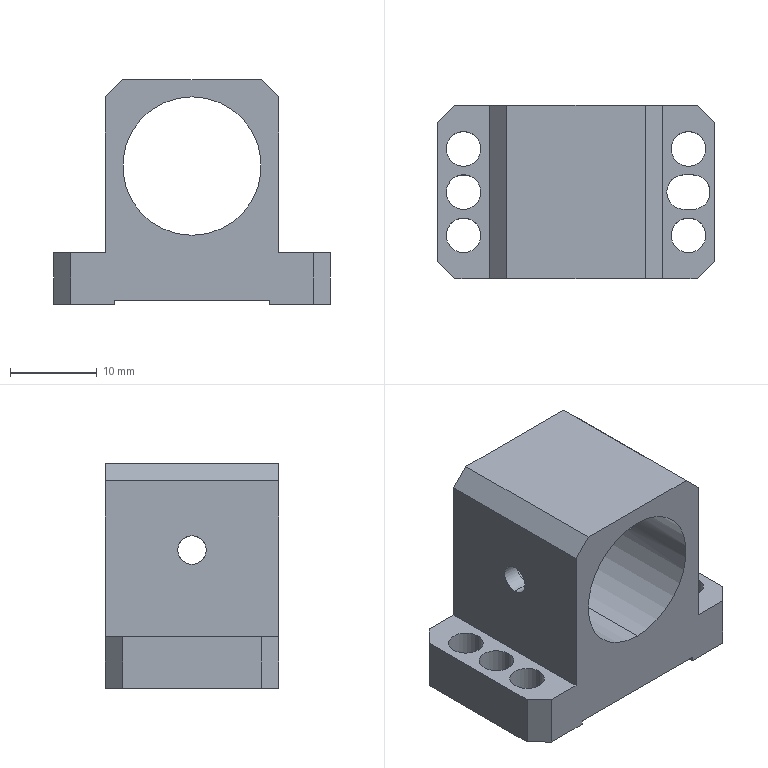NC program | NX | posted with a generic post | part box 32 x 20 x 26 mm
Lines 232 to 1055 of 2499:
(ZLEVEL_PROFILE_COPY_COPY_1 , TOOL : D3)
N444 T03 M6
N446 G54
N448 G17 G0 G90 X-13.314 Y-0.263 B0. C0. S9500 M3
N450 G43 Z30. H3
N452 Z1.
N454 G94 G1 X-13.242 Y-0.319 Z0.995 F1000.
N456 X-13.17 Y-0.373 Z0.99
N458 X-13.003 Y-0.41 Z0.982
N460 X-12.836 Y-0.376 Z0.973
N462 X-12.754 Y-0.316 Z0.967
N464 X-12.683 Y-0.26 Z0.963
N466 X-12.666 Y-0.237 Z0.961
N468 X-12.631 Y-0.154 Z0.956
N470 X-12.637 Y-0.109 Z0.954
N472 X-12.607 Y-0.077 Z0.952
N474 X-12.599 Y-0.036 Z0.949
N476 X-12.601 Y0.078 Z0.943
N478 X-12.63 Y0.152 Z0.939
N480 X-12.664 Y0.235 Z0.935
N482 X-12.828 Y0.372 Z0.923
N484 X-13.038 Y0.408 Z0.912
N486 X-13.209 Y0.353 Z0.903
N488 X-13.334 Y0.238 Z0.894
N490 X-13.402 Y0.082 Z0.885
N492 X-13.399 Y-0.079 Z0.877
N494 X-13.367 Y-0.159 Z0.872
N496 X-13.331 Y-0.242 Z0.867
N498 X-13.317 Y-0.26 Z0.866
N500 X-13.242 Y-0.319 Z0.861
N502 X-13.17 Y-0.373 Z0.856
N504 X-13.003 Y-0.41 Z0.847
N506 X-12.836 Y-0.376 Z0.838
N508 X-12.754 Y-0.316 Z0.833
N510 X-12.683 Y-0.26 Z0.828
N512 X-12.666 Y-0.237 Z0.827
N514 X-12.631 Y-0.154 Z0.822
N516 X-12.637 Y-0.109 Z0.82
N518 X-12.607 Y-0.077 Z0.818
N520 X-12.599 Y-0.036 Z0.815
N522 X-12.601 Y0.078 Z0.809
N524 X-12.63 Y0.152 Z0.805
N526 X-12.664 Y0.235 Z0.8
N528 X-12.828 Y0.372 Z0.789
N530 X-13.038 Y0.408 Z0.778
N532 X-13.209 Y0.353 Z0.769
N534 X-13.334 Y0.238 Z0.76
N536 X-13.402 Y0.082 Z0.751
N538 X-13.399 Y-0.079 Z0.742
N540 X-13.367 Y-0.159 Z0.738
N542 X-13.331 Y-0.242 Z0.733
N544 X-13.317 Y-0.26 Z0.732
N546 X-13.242 Y-0.319 Z0.727
N548 X-13.17 Y-0.373 Z0.722
N550 X-13.003 Y-0.41 Z0.713
N552 X-12.836 Y-0.376 Z0.704
N554 X-12.754 Y-0.316 Z0.699
N556 X-12.683 Y-0.26 Z0.694
N558 X-12.666 Y-0.237 Z0.693
N560 X-12.631 Y-0.154 Z0.688
N562 X-12.637 Y-0.109 Z0.686
N564 X-12.607 Y-0.077 Z0.683
N566 X-12.599 Y-0.036 Z0.681
N568 X-12.601 Y0.078 Z0.675
N570 X-12.63 Y0.152 Z0.671
N572 X-12.664 Y0.235 Z0.666
N574 X-12.828 Y0.372 Z0.655
N576 X-13.038 Y0.408 Z0.644
N578 X-13.209 Y0.353 Z0.635
N580 X-13.334 Y0.238 Z0.626
N582 X-13.402 Y0.082 Z0.617
N584 X-13.399 Y-0.079 Z0.608
N586 X-13.367 Y-0.159 Z0.604
N588 X-13.331 Y-0.242 Z0.599
N590 X-13.317 Y-0.26 Z0.598
N592 X-13.242 Y-0.319 Z0.593
N594 X-13.17 Y-0.373 Z0.588
N596 X-13.003 Y-0.41 Z0.579
N598 X-12.836 Y-0.376 Z0.57
N600 X-12.754 Y-0.316 Z0.565
N602 X-12.683 Y-0.26 Z0.56
N604 X-12.666 Y-0.237 Z0.559
N606 X-12.631 Y-0.154 Z0.554
N608 X-12.637 Y-0.109 Z0.552
N610 X-12.607 Y-0.077 Z0.549
N612 X-12.599 Y-0.036 Z0.547
N614 X-12.601 Y0.078 Z0.541
N616 X-12.63 Y0.152 Z0.537
N618 X-12.664 Y0.235 Z0.532
N620 X-12.828 Y0.372 Z0.521
N622 X-13.038 Y0.408 Z0.51
N624 X-13.209 Y0.353 Z0.5
N626 X-13.334 Y0.238 Z0.492
N628 X-13.402 Y0.082 Z0.483
N630 X-13.399 Y-0.079 Z0.474
N632 X-13.367 Y-0.159 Z0.47
N634 X-13.331 Y-0.242 Z0.465
N636 X-13.317 Y-0.26 Z0.464
N638 X-13.242 Y-0.319 Z0.459
N640 X-13.17 Y-0.373 Z0.454
N642 X-13.003 Y-0.41 Z0.445
N644 X-12.836 Y-0.376 Z0.436
N646 X-12.754 Y-0.316 Z0.431
N648 X-12.683 Y-0.26 Z0.426
N650 X-12.666 Y-0.237 Z0.425
N652 X-12.631 Y-0.154 Z0.42
N654 X-12.637 Y-0.109 Z0.418
N656 X-12.607 Y-0.077 Z0.415
N658 X-12.599 Y-0.036 Z0.413
N660 X-12.601 Y0.078 Z0.407
N662 X-12.63 Y0.152 Z0.403
N664 X-12.664 Y0.235 Z0.398
N666 X-12.828 Y0.372 Z0.387
N668 X-13.038 Y0.408 Z0.376
N670 X-13.209 Y0.353 Z0.366
N672 X-13.334 Y0.238 Z0.358
N674 X-13.402 Y0.082 Z0.349
N676 X-13.399 Y-0.079 Z0.34
N678 X-13.367 Y-0.159 Z0.336
N680 X-13.331 Y-0.242 Z0.331
N682 X-13.317 Y-0.26 Z0.33
N684 X-13.242 Y-0.319 Z0.325
N686 X-13.17 Y-0.373 Z0.32
N688 X-13.003 Y-0.41 Z0.311
N690 X-12.836 Y-0.376 Z0.302
N692 X-12.754 Y-0.316 Z0.297
N694 X-12.683 Y-0.26 Z0.292
N696 X-12.666 Y-0.237 Z0.291
N698 X-12.631 Y-0.154 Z0.286
N700 X-12.637 Y-0.109 Z0.283
N702 X-12.607 Y-0.077 Z0.281
N704 X-12.599 Y-0.036 Z0.279
N706 X-12.601 Y0.078 Z0.273
N708 X-12.63 Y0.152 Z0.269
N710 X-12.664 Y0.235 Z0.264
N712 X-12.828 Y0.372 Z0.253
N714 X-13.038 Y0.408 Z0.242
N716 X-13.209 Y0.353 Z0.232
N718 X-13.334 Y0.238 Z0.223
N720 X-13.402 Y0.082 Z0.215
N722 X-13.399 Y-0.079 Z0.206
N724 X-13.367 Y-0.159 Z0.202
N726 X-13.331 Y-0.242 Z0.197
N728 X-13.317 Y-0.26 Z0.196
N730 X-13.242 Y-0.319 Z0.191
N732 X-13.17 Y-0.373 Z0.186
N734 X-13.003 Y-0.41 Z0.177
N736 X-12.836 Y-0.376 Z0.168
N738 X-12.754 Y-0.316 Z0.163
N740 X-12.683 Y-0.26 Z0.158
N742 X-12.666 Y-0.237 Z0.156
N744 X-12.631 Y-0.154 Z0.152
N746 X-12.637 Y-0.109 Z0.149
N748 X-12.607 Y-0.077 Z0.147
N750 X-12.599 Y-0.036 Z0.145
N752 X-12.601 Y0.078 Z0.139
N754 X-12.63 Y0.152 Z0.135
N756 X-12.664 Y0.235 Z0.13
N758 X-12.828 Y0.372 Z0.119
N760 X-13.038 Y0.408 Z0.108
N762 X-13.209 Y0.353 Z0.098
N764 X-13.334 Y0.238 Z0.089
N766 X-13.402 Y0.082 Z0.08
N768 X-13.399 Y-0.079 Z0.072
N770 X-13.367 Y-0.159 Z0.067
N772 X-13.331 Y-0.242 Z0.063
N774 X-13.317 Y-0.26 Z0.062
N776 X-13.242 Y-0.319 Z0.057
N778 X-13.17 Y-0.373 Z0.052
N780 X-13.003 Y-0.41 Z0.043
N782 X-12.836 Y-0.376 Z0.034
N784 X-12.754 Y-0.316 Z0.029
N786 X-12.683 Y-0.26 Z0.024
N788 X-12.666 Y-0.237 Z0.022
N790 X-12.631 Y-0.154 Z0.018
N792 X-12.637 Y-0.109 Z0.015
N794 X-12.607 Y-0.077 Z0.013
N796 X-12.599 Y-0.036 Z0.011
N798 X-12.601 Y0.078 Z0.005
N800 X-12.63 Y0.152 Z0.001
N802 X-12.664 Y0.235 Z-0.004
N804 X-12.828 Y0.372 Z-0.015
N806 X-13.038 Y0.408 Z-0.026
N808 X-13.209 Y0.353 Z-0.036
N810 X-13.334 Y0.238 Z-0.045
N812 X-13.402 Y0.082 Z-0.054
N814 X-13.399 Y-0.079 Z-0.062
N816 X-13.367 Y-0.159 Z-0.067
N818 X-13.331 Y-0.242 Z-0.071
N820 X-13.317 Y-0.26 Z-0.073
N822 X-13.242 Y-0.319 Z-0.078
N824 X-13.17 Y-0.373 Z-0.082
N826 X-13.003 Y-0.41 Z-0.091
N828 X-12.836 Y-0.376 Z-0.1
N830 X-12.754 Y-0.316 Z-0.106
N832 X-12.683 Y-0.26 Z-0.11
N834 X-12.666 Y-0.237 Z-0.112
N836 X-12.631 Y-0.154 Z-0.116
N838 X-12.637 Y-0.109 Z-0.119
N840 X-12.607 Y-0.077 Z-0.121
N842 X-12.599 Y-0.036 Z-0.123
N844 X-12.601 Y0.078 Z-0.129
N846 X-12.63 Y0.152 Z-0.134
N848 X-12.664 Y0.235 Z-0.138
N850 X-12.828 Y0.372 Z-0.149
N852 X-13.038 Y0.408 Z-0.161
N854 X-13.209 Y0.353 Z-0.17
N856 X-13.334 Y0.238 Z-0.179
N858 X-13.402 Y0.082 Z-0.188
N860 X-13.399 Y-0.079 Z-0.196
N862 X-13.372 Y-0.146 Z-0.2
N864 X-13.367 Y-0.159 F1200.
N866 G3 X-12.631 Y-0.154 R0.4
N868 G1 X-12.641 Y-0.125
N870 X-12.632 Y-0.096
N872 X-12.607 Y-0.077
N874 G3 X-13.372 Y-0.146 R-0.4
N876 G1 X-13.319 Y-0.228 Z-0.21
N878 X-13.269 Y-0.286 Z-0.219
N880 X-13.224 Y-0.322 Z-0.225
N882 X-13.139 Y-0.366 Z-0.235
N884 X-13.095 Y-0.381 Z-0.24
N886 X-13.066 Y-0.387 Z-0.243
N888 X-13.007 Y-0.392 Z-0.25
N890 X-12.912 Y-0.382 Z-0.26
N892 X-12.868 Y-0.369 Z-0.265
N894 X-12.84 Y-0.358 Z-0.268
N896 X-12.788 Y-0.33 Z-0.275
N898 X-12.715 Y-0.269 Z-0.285
N900 X-12.685 Y-0.234 Z-0.29
N902 X-12.668 Y-0.209 Z-0.293
N904 X-12.64 Y-0.156 Z-0.3
N906 X-12.613 Y-0.066 Z-0.31
N908 X-12.608 Y-0.021 Z-0.315
N910 X-12.607 Y0.009 Z-0.318
N912 X-12.614 Y0.068 Z-0.325
N914 X-12.642 Y0.159 Z-0.335
N916 X-12.663 Y0.2 Z-0.34
N918 X-12.679 Y0.225 Z-0.343
N920 X-12.717 Y0.271 Z-0.35
N922 X-12.789 Y0.33 Z-0.36
N924 X-12.828 Y0.352 Z-0.365
N926 X-12.856 Y0.365 Z-0.368
N928 X-12.915 Y0.383 Z-0.375
N930 X-12.974 Y0.391 Z-0.381
N932 X-13.031 Z-0.388
N934 X-13.089 Y0.383 Z-0.394
N936 X-13.145 Y0.373 Z-0.4
N938 G3 X-13.372 Y-0.146 R0.4
N940 G1 X-13.319 Y-0.228 Z-0.41
N942 X-13.269 Y-0.286 Z-0.419
N944 X-13.224 Y-0.322 Z-0.425
N946 X-13.139 Y-0.366 Z-0.435
N948 X-13.095 Y-0.381 Z-0.44
N950 X-13.066 Y-0.387 Z-0.443
N952 X-13.007 Y-0.392 Z-0.45
N954 X-12.912 Y-0.382 Z-0.46
N956 X-12.868 Y-0.369 Z-0.465
N958 X-12.84 Y-0.358 Z-0.468
N960 X-12.788 Y-0.33 Z-0.475
N962 X-12.715 Y-0.269 Z-0.485
N964 X-12.685 Y-0.234 Z-0.49
N966 X-12.668 Y-0.209 Z-0.493
N968 X-12.64 Y-0.156 Z-0.5
N970 X-12.613 Y-0.066 Z-0.51
N972 X-12.608 Y-0.021 Z-0.515
N974 X-12.607 Y0.009 Z-0.518
N976 X-12.614 Y0.068 Z-0.525
N978 X-12.642 Y0.159 Z-0.535
N980 X-12.663 Y0.2 Z-0.54
N982 X-12.679 Y0.225 Z-0.543
N984 X-12.717 Y0.271 Z-0.55
N986 X-12.789 Y0.33 Z-0.56
N988 X-12.828 Y0.352 Z-0.565
N990 X-12.856 Y0.365 Z-0.568
N992 X-12.915 Y0.383 Z-0.575
N994 X-12.974 Y0.391 Z-0.581
N996 X-13.031 Z-0.588
N998 X-13.089 Y0.383 Z-0.594
N1000 X-13.145 Y0.373 Z-0.6
N1002 G3 X-13.372 Y-0.146 R0.4
N1004 G1 X-13.319 Y-0.228 Z-0.61
N1006 X-13.269 Y-0.286 Z-0.619
N1008 X-13.224 Y-0.322 Z-0.625
N1010 X-13.139 Y-0.366 Z-0.635
N1012 X-13.095 Y-0.381 Z-0.64
N1014 X-13.066 Y-0.387 Z-0.643
N1016 X-13.007 Y-0.392 Z-0.65
N1018 X-12.912 Y-0.382 Z-0.66
N1020 X-12.868 Y-0.369 Z-0.665
N1022 X-12.84 Y-0.358 Z-0.668
N1024 X-12.788 Y-0.33 Z-0.675
N1026 X-12.715 Y-0.269 Z-0.685
N1028 X-12.685 Y-0.234 Z-0.69
N1030 X-12.668 Y-0.209 Z-0.693
N1032 X-12.64 Y-0.156 Z-0.7
N1034 X-12.613 Y-0.066 Z-0.71
N1036 X-12.608 Y-0.021 Z-0.715
N1038 X-12.607 Y0.009 Z-0.718
N1040 X-12.614 Y0.068 Z-0.725
N1042 X-12.642 Y0.159 Z-0.735
N1044 X-12.663 Y0.2 Z-0.74
N1046 X-12.679 Y0.225 Z-0.743
N1048 X-12.717 Y0.271 Z-0.75
N1050 X-12.789 Y0.33 Z-0.76
N1052 X-12.828 Y0.352 Z-0.765
N1054 X-12.856 Y0.365 Z-0.768
N1056 X-12.915 Y0.383 Z-0.775
N1058 X-12.974 Y0.391 Z-0.781
N1060 X-13.031 Z-0.788
N1062 X-13.089 Y0.383 Z-0.794
N1064 X-13.145 Y0.373 Z-0.8
N1066 G3 X-13.372 Y-0.146 R0.4
N1068 G1 X-13.319 Y-0.228 Z-0.81
N1070 X-13.269 Y-0.286 Z-0.819
N1072 X-13.224 Y-0.322 Z-0.825
N1074 X-13.139 Y-0.366 Z-0.835
N1076 X-13.095 Y-0.381 Z-0.84
N1078 X-13.066 Y-0.387 Z-0.843
N1080 X-13.007 Y-0.392 Z-0.85
N1082 X-12.912 Y-0.382 Z-0.86
N1084 X-12.868 Y-0.369 Z-0.865
N1086 X-12.84 Y-0.358 Z-0.868
N1088 X-12.788 Y-0.33 Z-0.875
N1090 X-12.715 Y-0.269 Z-0.885
N1092 X-12.685 Y-0.234 Z-0.89
N1094 X-12.668 Y-0.209 Z-0.893
N1096 X-12.64 Y-0.156 Z-0.9
N1098 X-12.613 Y-0.066 Z-0.91
N1100 X-12.608 Y-0.021 Z-0.915
N1102 X-12.607 Y0.009 Z-0.918
N1104 X-12.614 Y0.068 Z-0.925
N1106 X-12.642 Y0.159 Z-0.935
N1108 X-12.663 Y0.2 Z-0.94
N1110 X-12.679 Y0.225 Z-0.943
N1112 X-12.717 Y0.271 Z-0.95
N1114 X-12.789 Y0.33 Z-0.96
N1116 X-12.828 Y0.352 Z-0.965
N1118 X-12.856 Y0.365 Z-0.968
N1120 X-12.915 Y0.383 Z-0.975
N1122 X-12.974 Y0.391 Z-0.981
N1124 X-13.031 Z-0.988
N1126 X-13.089 Y0.383 Z-0.994
N1128 X-13.145 Y0.373 Z-1.
N1130 G3 X-13.372 Y-0.146 R0.4
N1132 G1 X-13.319 Y-0.228 Z-1.01
N1134 X-13.269 Y-0.286 Z-1.019
N1136 X-13.224 Y-0.322 Z-1.025
N1138 X-13.139 Y-0.366 Z-1.035
N1140 X-13.095 Y-0.381 Z-1.04
N1142 X-13.066 Y-0.387 Z-1.043
N1144 X-13.007 Y-0.392 Z-1.05
N1146 X-12.912 Y-0.382 Z-1.06
N1148 X-12.868 Y-0.369 Z-1.065
N1150 X-12.84 Y-0.358 Z-1.068
N1152 X-12.788 Y-0.33 Z-1.075
N1154 X-12.715 Y-0.269 Z-1.085
N1156 X-12.685 Y-0.234 Z-1.09
N1158 X-12.668 Y-0.209 Z-1.093
N1160 X-12.64 Y-0.156 Z-1.1
N1162 X-12.613 Y-0.066 Z-1.11
N1164 X-12.608 Y-0.021 Z-1.115
N1166 X-12.607 Y0.009 Z-1.118
N1168 X-12.614 Y0.068 Z-1.125
N1170 X-12.642 Y0.159 Z-1.135
N1172 X-12.663 Y0.2 Z-1.14
N1174 X-12.679 Y0.225 Z-1.143
N1176 X-12.717 Y0.271 Z-1.15
N1178 X-12.789 Y0.33 Z-1.16
N1180 X-12.828 Y0.352 Z-1.165
N1182 X-12.856 Y0.365 Z-1.168
N1184 X-12.915 Y0.383 Z-1.175
N1186 X-12.974 Y0.391 Z-1.181
N1188 X-13.031 Z-1.188
N1190 X-13.089 Y0.383 Z-1.194
N1192 X-13.145 Y0.373 Z-1.2
N1194 G3 X-13.372 Y-0.146 R0.4
N1196 G1 X-13.319 Y-0.228 Z-1.21
N1198 X-13.269 Y-0.286 Z-1.219
N1200 X-13.224 Y-0.322 Z-1.225
N1202 X-13.139 Y-0.366 Z-1.235
N1204 X-13.095 Y-0.381 Z-1.24
N1206 X-13.066 Y-0.387 Z-1.243
N1208 X-13.007 Y-0.392 Z-1.25
N1210 X-12.912 Y-0.382 Z-1.26
N1212 X-12.868 Y-0.369 Z-1.265
N1214 X-12.84 Y-0.358 Z-1.268
N1216 X-12.788 Y-0.33 Z-1.275
N1218 X-12.715 Y-0.269 Z-1.285
N1220 X-12.685 Y-0.234 Z-1.29
N1222 X-12.668 Y-0.209 Z-1.293
N1224 X-12.64 Y-0.156 Z-1.3
N1226 X-12.613 Y-0.066 Z-1.31
N1228 X-12.608 Y-0.021 Z-1.315
N1230 Y0.009 Z-1.318
N1232 X-12.614 Y0.068 Z-1.325
N1234 X-12.642 Y0.159 Z-1.335
N1236 X-12.663 Y0.2 Z-1.34
N1238 X-12.679 Y0.225 Z-1.343
N1240 X-12.717 Y0.271 Z-1.35
N1242 X-12.789 Y0.33 Z-1.36
N1244 X-12.828 Y0.352 Z-1.365
N1246 X-12.856 Y0.365 Z-1.368
N1248 X-12.915 Y0.383 Z-1.375
N1250 X-12.974 Y0.391 Z-1.381
N1252 X-13.031 Z-1.388
N1254 X-13.089 Y0.383 Z-1.394
N1256 X-13.145 Y0.373 Z-1.4
N1258 G3 X-13.372 Y-0.146 R0.4
N1260 G1 X-13.319 Y-0.228 Z-1.41
N1262 X-13.269 Y-0.286 Z-1.419
N1264 X-13.224 Y-0.322 Z-1.425
N1266 X-13.139 Y-0.366 Z-1.435
N1268 X-13.095 Y-0.38 Z-1.44
N1270 X-13.066 Y-0.387 Z-1.443
N1272 X-13.007 Y-0.392 Z-1.45
N1274 X-12.912 Y-0.382 Z-1.46
N1276 X-12.868 Y-0.369 Z-1.465
N1278 X-12.84 Y-0.358 Z-1.468
N1280 X-12.788 Y-0.33 Z-1.475
N1282 X-12.715 Y-0.269 Z-1.485
N1284 X-12.685 Y-0.234 Z-1.49
N1286 X-12.668 Y-0.209 Z-1.493
N1288 X-12.64 Y-0.156 Z-1.5
N1290 X-12.613 Y-0.066 Z-1.51
N1292 X-12.608 Y-0.021 Z-1.515
N1294 Y0.009 Z-1.518
N1296 X-12.614 Y0.068 Z-1.525
N1298 X-12.642 Y0.159 Z-1.535
N1300 X-12.663 Y0.2 Z-1.54
N1302 X-12.679 Y0.225 Z-1.543
N1304 X-12.717 Y0.271 Z-1.55
N1306 X-12.789 Y0.33 Z-1.56
N1308 X-12.828 Y0.352 Z-1.565
N1310 X-12.856 Y0.365 Z-1.568
N1312 X-12.915 Y0.383 Z-1.575
N1314 X-12.974 Y0.391 Z-1.581
N1316 X-13.031 Z-1.588
N1318 X-13.089 Y0.383 Z-1.594
N1320 X-13.145 Y0.373 Z-1.6
N1322 G3 X-13.372 Y-0.146 R0.4
N1324 G1 X-13.319 Y-0.228 Z-1.61
N1326 X-13.269 Y-0.286 Z-1.619
N1328 X-13.224 Y-0.322 Z-1.625
N1330 X-13.139 Y-0.366 Z-1.635
N1332 X-13.095 Y-0.38 Z-1.64
N1334 X-13.066 Y-0.387 Z-1.643
N1336 X-13.007 Y-0.392 Z-1.65
N1338 X-12.912 Y-0.382 Z-1.66
N1340 X-12.868 Y-0.369 Z-1.665
N1342 X-12.84 Y-0.358 Z-1.668
N1344 X-12.788 Y-0.33 Z-1.675
N1346 X-12.715 Y-0.269 Z-1.685
N1348 X-12.685 Y-0.234 Z-1.69
N1350 X-12.668 Y-0.209 Z-1.693
N1352 X-12.64 Y-0.156 Z-1.7
N1354 X-12.613 Y-0.066 Z-1.71
N1356 X-12.608 Y-0.021 Z-1.715
N1358 Y0.009 Z-1.718
N1360 X-12.614 Y0.068 Z-1.725
N1362 X-12.642 Y0.159 Z-1.735
N1364 X-12.663 Y0.2 Z-1.74
N1366 X-12.679 Y0.225 Z-1.743
N1368 X-12.717 Y0.271 Z-1.75
N1370 X-12.789 Y0.33 Z-1.76
N1372 X-12.828 Y0.352 Z-1.765
N1374 X-12.856 Y0.365 Z-1.768
N1376 X-12.915 Y0.383 Z-1.775
N1378 X-12.974 Y0.391 Z-1.781
N1380 X-13.031 Z-1.788
N1382 X-13.089 Y0.383 Z-1.794
N1384 X-13.145 Y0.373 Z-1.8
N1386 G3 X-13.372 Y-0.146 R0.4
N1388 G1 X-13.319 Y-0.228 Z-1.81
N1390 X-13.269 Y-0.286 Z-1.819
N1392 X-13.224 Y-0.322 Z-1.825
N1394 X-13.139 Y-0.366 Z-1.835
N1396 X-13.095 Y-0.38 Z-1.84
N1398 X-13.066 Y-0.387 Z-1.843
N1400 X-13.007 Y-0.392 Z-1.85
N1402 X-12.912 Y-0.382 Z-1.86
N1404 X-12.868 Y-0.369 Z-1.865
N1406 X-12.84 Y-0.358 Z-1.868
N1408 X-12.788 Y-0.33 Z-1.875
N1410 X-12.715 Y-0.269 Z-1.885
N1412 X-12.685 Y-0.234 Z-1.89
N1414 X-12.668 Y-0.209 Z-1.893
N1416 X-12.64 Y-0.156 Z-1.9
N1418 X-12.613 Y-0.066 Z-1.91
N1420 X-12.608 Y-0.021 Z-1.915
N1422 Y0.009 Z-1.918
N1424 X-12.614 Y0.068 Z-1.925
N1426 X-12.642 Y0.159 Z-1.935
N1428 X-12.663 Y0.2 Z-1.94
N1430 X-12.679 Y0.225 Z-1.943
N1432 X-12.717 Y0.271 Z-1.95
N1434 X-12.789 Y0.33 Z-1.96
N1436 X-12.828 Y0.352 Z-1.965
N1438 X-12.856 Y0.365 Z-1.968
N1440 X-12.915 Y0.383 Z-1.975
N1442 X-12.974 Y0.391 Z-1.981
N1444 X-13.031 Z-1.988
N1446 X-13.089 Y0.383 Z-1.994
N1448 X-13.145 Y0.373 Z-2.
N1450 G3 X-13.372 Y-0.146 R0.4
N1452 G1 X-13.319 Y-0.228 Z-2.01
N1454 X-13.269 Y-0.286 Z-2.019
N1456 X-13.224 Y-0.322 Z-2.025
N1458 X-13.139 Y-0.366 Z-2.035
N1460 X-13.095 Y-0.38 Z-2.04
N1462 X-13.066 Y-0.387 Z-2.043
N1464 X-13.007 Y-0.392 Z-2.05
N1466 X-12.912 Y-0.382 Z-2.06
N1468 X-12.868 Y-0.369 Z-2.065
N1470 X-12.84 Y-0.358 Z-2.068
N1472 X-12.788 Y-0.33 Z-2.075
N1474 X-12.715 Y-0.269 Z-2.085
N1476 X-12.685 Y-0.234 Z-2.09
N1478 X-12.668 Y-0.209 Z-2.093
N1480 X-12.64 Y-0.156 Z-2.1
N1482 X-12.613 Y-0.066 Z-2.11
N1484 X-12.608 Y-0.021 Z-2.115
N1486 Y0.009 Z-2.118
N1488 X-12.614 Y0.068 Z-2.125
N1490 X-12.642 Y0.159 Z-2.135
N1492 X-12.663 Y0.2 Z-2.14
N1494 X-12.679 Y0.225 Z-2.143
N1496 X-12.717 Y0.271 Z-2.15
N1498 X-12.789 Y0.33 Z-2.16
N1500 X-12.828 Y0.352 Z-2.165
N1502 X-12.856 Y0.365 Z-2.168
N1504 X-12.915 Y0.383 Z-2.175
N1506 X-12.974 Y0.391 Z-2.181
N1508 X-13.031 Z-2.188
N1510 X-13.089 Y0.383 Z-2.194
N1512 X-13.145 Y0.373 Z-2.2
N1514 G3 X-13.372 Y-0.146 R0.4
N1516 G1 X-13.319 Y-0.228 Z-2.21
N1518 X-13.269 Y-0.286 Z-2.219
N1520 X-13.224 Y-0.322 Z-2.225
N1522 X-13.139 Y-0.366 Z-2.235
N1524 X-13.095 Y-0.38 Z-2.24
N1526 X-13.066 Y-0.387 Z-2.243
N1528 X-13.007 Y-0.392 Z-2.25
N1530 X-12.912 Y-0.382 Z-2.26
N1532 X-12.868 Y-0.369 Z-2.265
N1534 X-12.84 Y-0.358 Z-2.268
N1536 X-12.788 Y-0.33 Z-2.275
N1538 X-12.715 Y-0.269 Z-2.285
N1540 X-12.685 Y-0.234 Z-2.29
N1542 X-12.668 Y-0.209 Z-2.293
N1544 X-12.64 Y-0.156 Z-2.3
N1546 X-12.613 Y-0.066 Z-2.31
N1548 X-12.608 Y-0.021 Z-2.315
N1550 Y0.009 Z-2.318
N1552 X-12.614 Y0.068 Z-2.325
N1554 X-12.642 Y0.159 Z-2.335
N1556 X-12.663 Y0.2 Z-2.34
N1558 X-12.679 Y0.225 Z-2.343
N1560 X-12.717 Y0.271 Z-2.35
N1562 X-12.789 Y0.33 Z-2.36
N1564 X-12.828 Y0.352 Z-2.365
N1566 X-12.856 Y0.365 Z-2.368
N1568 X-12.915 Y0.383 Z-2.375
N1570 X-12.974 Y0.391 Z-2.381
N1572 X-13.031 Z-2.388
N1574 X-13.089 Y0.383 Z-2.394
N1576 X-13.145 Y0.373 Z-2.4
N1578 G3 X-13.372 Y-0.146 R0.4
N1580 G1 X-13.319 Y-0.228 Z-2.41
N1582 X-13.269 Y-0.286 Z-2.419
N1584 X-13.224 Y-0.322 Z-2.425
N1586 X-13.139 Y-0.366 Z-2.435
N1588 X-13.095 Y-0.38 Z-2.44
N1590 X-13.066 Y-0.387 Z-2.443
N1592 X-13.007 Y-0.392 Z-2.45
N1594 X-12.912 Y-0.382 Z-2.46
N1596 X-12.868 Y-0.369 Z-2.465
N1598 X-12.84 Y-0.358 Z-2.468
N1600 X-12.788 Y-0.33 Z-2.475
N1602 X-12.715 Y-0.269 Z-2.485
N1604 X-12.685 Y-0.234 Z-2.49
N1606 X-12.668 Y-0.209 Z-2.493
N1608 X-12.64 Y-0.156 Z-2.5
N1610 X-12.613 Y-0.066 Z-2.51
N1612 X-12.608 Y-0.021 Z-2.515
N1614 Y0.009 Z-2.518
N1616 X-12.614 Y0.068 Z-2.525
N1618 X-12.642 Y0.159 Z-2.535
N1620 X-12.663 Y0.2 Z-2.54
N1622 X-12.679 Y0.225 Z-2.543
N1624 X-12.717 Y0.271 Z-2.55
N1626 X-12.789 Y0.33 Z-2.56
N1628 X-12.828 Y0.352 Z-2.565
N1630 X-12.856 Y0.365 Z-2.568
N1632 X-12.915 Y0.383 Z-2.575
N1634 X-12.974 Y0.391 Z-2.581
N1636 X-13.031 Z-2.588
N1638 X-13.089 Y0.383 Z-2.594
N1640 X-13.145 Y0.373 Z-2.6
N1642 G3 X-13.372 Y-0.146 R0.4
N1644 G1 X-13.319 Y-0.228 Z-2.61
N1646 X-13.269 Y-0.286 Z-2.619
N1648 X-13.224 Y-0.322 Z-2.625
N1650 X-13.139 Y-0.366 Z-2.635
N1652 X-13.095 Y-0.38 Z-2.64
N1654 X-13.066 Y-0.387 Z-2.643
N1656 X-13.007 Y-0.392 Z-2.65
N1658 X-12.912 Y-0.382 Z-2.66
N1660 X-12.868 Y-0.369 Z-2.665
N1662 X-12.84 Y-0.358 Z-2.668
N1664 X-12.788 Y-0.33 Z-2.675
N1666 X-12.715 Y-0.269 Z-2.685
N1668 X-12.685 Y-0.234 Z-2.69
N1670 X-12.668 Y-0.209 Z-2.693
N1672 X-12.64 Y-0.156 Z-2.7
N1674 X-12.613 Y-0.066 Z-2.71
N1676 X-12.608 Y-0.021 Z-2.715
N1678 Y0.009 Z-2.718
N1680 X-12.614 Y0.068 Z-2.725
N1682 X-12.642 Y0.159 Z-2.735
N1684 X-12.663 Y0.2 Z-2.74
N1686 X-12.679 Y0.225 Z-2.743
N1688 X-12.717 Y0.271 Z-2.75
N1690 X-12.789 Y0.33 Z-2.76
N1692 X-12.828 Y0.352 Z-2.765
N1694 X-12.856 Y0.365 Z-2.768
N1696 X-12.915 Y0.383 Z-2.775
N1698 X-12.974 Y0.391 Z-2.781
N1700 X-13.031 Z-2.788
N1702 X-13.089 Y0.383 Z-2.794
N1704 X-13.145 Y0.373 Z-2.8
N1706 G3 X-13.372 Y-0.146 R0.4
N1708 G1 X-13.319 Y-0.228 Z-2.81
N1710 X-13.269 Y-0.286 Z-2.819
N1712 X-13.224 Y-0.322 Z-2.825
N1714 X-13.139 Y-0.366 Z-2.835
N1716 X-13.095 Y-0.38 Z-2.84
N1718 X-13.066 Y-0.387 Z-2.843
N1720 X-13.007 Y-0.392 Z-2.85
N1722 X-12.912 Y-0.382 Z-2.86
N1724 X-12.868 Y-0.369 Z-2.865
N1726 X-12.84 Y-0.358 Z-2.868
N1728 X-12.788 Y-0.33 Z-2.875
N1730 X-12.715 Y-0.269 Z-2.885
N1732 X-12.685 Y-0.234 Z-2.89
N1734 X-12.668 Y-0.209 Z-2.893
N1736 X-12.64 Y-0.156 Z-2.9
N1738 X-12.613 Y-0.066 Z-2.91
N1740 X-12.608 Y-0.021 Z-2.915
N1742 Y0.009 Z-2.918
N1744 X-12.614 Y0.068 Z-2.925
N1746 X-12.642 Y0.159 Z-2.935
N1748 X-12.663 Y0.2 Z-2.94
N1750 X-12.679 Y0.225 Z-2.943
N1752 X-12.717 Y0.271 Z-2.95
N1754 X-12.789 Y0.33 Z-2.96
N1756 X-12.828 Y0.352 Z-2.965
N1758 X-12.856 Y0.365 Z-2.968
N1760 X-12.915 Y0.383 Z-2.975
N1762 X-12.974 Y0.391 Z-2.981
N1764 X-13.031 Z-2.988
N1766 X-13.089 Y0.383 Z-2.994
N1768 X-13.145 Y0.373 Z-3.
N1770 G3 X-13.372 Y-0.146 R0.4
N1772 G1 X-13.319 Y-0.228 Z-3.01
N1774 X-13.269 Y-0.286 Z-3.019
N1776 X-13.224 Y-0.322 Z-3.025
N1778 X-13.139 Y-0.366 Z-3.035
N1780 X-13.095 Y-0.38 Z-3.04
N1782 X-13.066 Y-0.387 Z-3.043
N1784 X-13.007 Y-0.392 Z-3.05
N1786 X-12.912 Y-0.382 Z-3.06
N1788 X-12.868 Y-0.369 Z-3.065
N1790 X-12.84 Y-0.358 Z-3.068
N1792 X-12.788 Y-0.33 Z-3.075
N1794 X-12.715 Y-0.269 Z-3.085
N1796 X-12.685 Y-0.234 Z-3.09
N1798 X-12.668 Y-0.209 Z-3.093
N1800 X-12.64 Y-0.156 Z-3.1
N1802 X-12.613 Y-0.066 Z-3.11
N1804 X-12.608 Y-0.021 Z-3.115
N1806 Y0.009 Z-3.118
N1808 X-12.614 Y0.068 Z-3.125
N1810 X-12.642 Y0.159 Z-3.135
N1812 X-12.663 Y0.2 Z-3.14
N1814 X-12.679 Y0.225 Z-3.143
N1816 X-12.717 Y0.271 Z-3.15
N1818 X-12.789 Y0.33 Z-3.16
N1820 X-12.828 Y0.352 Z-3.165
N1822 X-12.856 Y0.365 Z-3.168
N1824 X-12.915 Y0.383 Z-3.175
N1826 X-12.974 Y0.391 Z-3.181
N1828 X-13.031 Z-3.188
N1830 X-13.089 Y0.383 Z-3.194
N1832 X-13.145 Y0.373 Z-3.2
N1834 G3 X-13.372 Y-0.146 R0.4
N1836 G1 X-13.319 Y-0.228 Z-3.21
N1838 X-13.269 Y-0.286 Z-3.219
N1840 X-13.224 Y-0.322 Z-3.225
N1842 X-13.139 Y-0.366 Z-3.235
N1844 X-13.095 Y-0.38 Z-3.24
N1846 X-13.066 Y-0.387 Z-3.243
N1848 X-13.007 Y-0.392 Z-3.25
N1850 X-12.912 Y-0.382 Z-3.26
N1852 X-12.868 Y-0.369 Z-3.265
N1854 X-12.84 Y-0.358 Z-3.268
N1856 X-12.788 Y-0.33 Z-3.275
N1858 X-12.715 Y-0.269 Z-3.285
N1860 X-12.685 Y-0.234 Z-3.29
N1862 X-12.668 Y-0.209 Z-3.293
N1864 X-12.64 Y-0.156 Z-3.3
N1866 X-12.613 Y-0.066 Z-3.31
N1868 X-12.608 Y-0.021 Z-3.315
N1870 Y0.009 Z-3.318
N1872 X-12.614 Y0.068 Z-3.325
N1874 X-12.642 Y0.159 Z-3.335
N1876 X-12.663 Y0.2 Z-3.34
N1878 X-12.679 Y0.225 Z-3.343
N1880 X-12.717 Y0.271 Z-3.35
N1882 X-12.789 Y0.33 Z-3.36
N1884 X-12.828 Y0.352 Z-3.365
N1886 X-12.856 Y0.365 Z-3.368
N1888 X-12.915 Y0.383 Z-3.375
N1890 X-12.974 Y0.391 Z-3.381
N1892 X-13.031 Z-3.388
N1894 X-13.089 Y0.383 Z-3.394
N1896 X-13.145 Y0.373 Z-3.4
N1898 G3 X-13.372 Y-0.146 R0.4
N1900 G1 X-13.319 Y-0.228 Z-3.41
N1902 X-13.269 Y-0.286 Z-3.419
N1904 X-13.224 Y-0.322 Z-3.425
N1906 X-13.139 Y-0.366 Z-3.435
N1908 X-13.095 Y-0.38 Z-3.44
N1910 X-13.066 Y-0.387 Z-3.443
N1912 X-13.007 Y-0.392 Z-3.45
N1914 X-12.912 Y-0.382 Z-3.46
N1916 X-12.868 Y-0.369 Z-3.465
N1918 X-12.84 Y-0.358 Z-3.468
N1920 X-12.788 Y-0.33 Z-3.475
N1922 X-12.715 Y-0.269 Z-3.485
N1924 X-12.685 Y-0.234 Z-3.49
N1926 X-12.668 Y-0.209 Z-3.493
N1928 X-12.64 Y-0.156 Z-3.5
N1930 X-12.613 Y-0.066 Z-3.51
N1932 X-12.608 Y-0.021 Z-3.515
N1934 Y0.009 Z-3.518
N1936 X-12.614 Y0.068 Z-3.525
N1938 X-12.642 Y0.159 Z-3.535
N1940 X-12.663 Y0.2 Z-3.54
N1942 X-12.679 Y0.225 Z-3.543
N1944 X-12.717 Y0.271 Z-3.55
N1946 X-12.789 Y0.33 Z-3.56
N1948 X-12.828 Y0.352 Z-3.565
N1950 X-12.856 Y0.365 Z-3.568
N1952 X-12.915 Y0.383 Z-3.575
N1954 X-12.974 Y0.391 Z-3.581
N1956 X-13.031 Z-3.588
N1958 X-13.089 Y0.383 Z-3.594
N1960 X-13.145 Y0.373 Z-3.6
N1962 G3 X-13.372 Y-0.146 R0.4
N1964 G1 X-13.319 Y-0.228 Z-3.61
N1966 X-13.269 Y-0.286 Z-3.619
N1968 X-13.224 Y-0.322 Z-3.625
N1970 X-13.139 Y-0.366 Z-3.635
N1972 X-13.095 Y-0.38 Z-3.64
N1974 X-13.066 Y-0.387 Z-3.643
N1976 X-13.007 Y-0.392 Z-3.65
N1978 X-12.912 Y-0.382 Z-3.66
N1980 X-12.868 Y-0.369 Z-3.665
N1982 X-12.84 Y-0.358 Z-3.668
N1984 X-12.788 Y-0.33 Z-3.675
N1986 X-12.715 Y-0.269 Z-3.685
N1988 X-12.685 Y-0.234 Z-3.69
N1990 X-12.668 Y-0.209 Z-3.693
N1992 X-12.64 Y-0.156 Z-3.7
N1994 X-12.613 Y-0.066 Z-3.71
N1996 X-12.608 Y-0.021 Z-3.715
N1998 Y0.009 Z-3.718
N2000 X-12.614 Y0.068 Z-3.725
N2002 X-12.642 Y0.159 Z-3.735
N2004 X-12.663 Y0.2 Z-3.74
N2006 X-12.679 Y0.225 Z-3.743
N2008 X-12.717 Y0.271 Z-3.75
N2010 X-12.789 Y0.33 Z-3.76
N2012 X-12.856 Y0.366 Z-3.768
N2014 X-12.915 Y0.383 Z-3.775
N2016 X-12.974 Y0.391 Z-3.781
N2018 X-13.031 Z-3.788
N2020 X-13.089 Y0.383 Z-3.794
N2022 X-13.145 Y0.373 Z-3.8
N2024 G3 X-13.372 Y-0.146 R0.4
N2026 G1 X-13.319 Y-0.228 Z-3.81
N2028 X-13.269 Y-0.286 Z-3.819
N2030 X-13.224 Y-0.322 Z-3.825
N2032 X-13.139 Y-0.366 Z-3.835
N2034 X-13.095 Y-0.38 Z-3.84
N2036 X-13.066 Y-0.387 Z-3.843
N2038 X-13.007 Y-0.392 Z-3.85
N2040 X-12.912 Y-0.382 Z-3.86
N2042 X-12.868 Y-0.369 Z-3.865
N2044 X-12.84 Y-0.358 Z-3.868
N2046 X-12.788 Y-0.33 Z-3.875
N2048 X-12.715 Y-0.269 Z-3.885
N2050 X-12.685 Y-0.234 Z-3.89
N2052 X-12.668 Y-0.209 Z-3.893
N2054 X-12.64 Y-0.156 Z-3.9
N2056 X-12.613 Y-0.066 Z-3.91
N2058 X-12.608 Y-0.021 Z-3.915
N2060 Y0.009 Z-3.918
N2062 X-12.614 Y0.068 Z-3.925
N2064 X-12.642 Y0.159 Z-3.935
N2066 X-12.663 Y0.2 Z-3.94
N2068 X-12.679 Y0.225 Z-3.943
N2070 X-12.717 Y0.271 Z-3.95
N2072 X-12.789 Y0.33 Z-3.96
N2074 X-12.856 Y0.366 Z-3.968
N2076 X-12.915 Y0.383 Z-3.975
N2078 X-12.974 Y0.391 Z-3.981
N2080 X-13.031 Z-3.988
N2082 X-13.089 Y0.383 Z-3.994
N2084 X-13.145 Y0.373 Z-4.